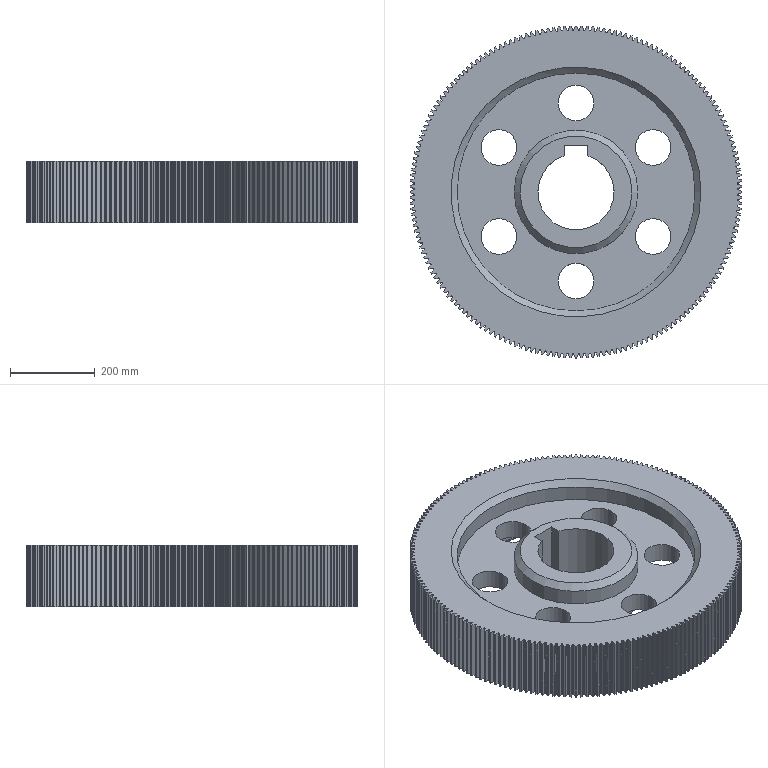Part | NX | features BREP 184, META 184, INSTANCE 55, EXTRUDE 6, SKETCH 4, CHAMFER 2, CYLINDER 2, DATUM_CSYS 2, Delete Body 2, EXTRACT_FACE 2, CIRCULAR_ISET 1, FSET 1, Instance Feature 1, LINKED_BODY 1, Mirror Feature 1, REPLACE_FACE 1, Resize Face 1, SCALE 1, SWP104 1, TRANSFORM_ISET 1 | 1 solid | 1128 faces | box 784.688 x 784.688 x 146.25 mm | volume 44829602 mm3 | spline 920 | cylinder 195 | plane 9 | cone 4 | commonest cylinder face diameters 765.703 x184 84.375 x6 292.5 x2 562.5 x2 180 x1